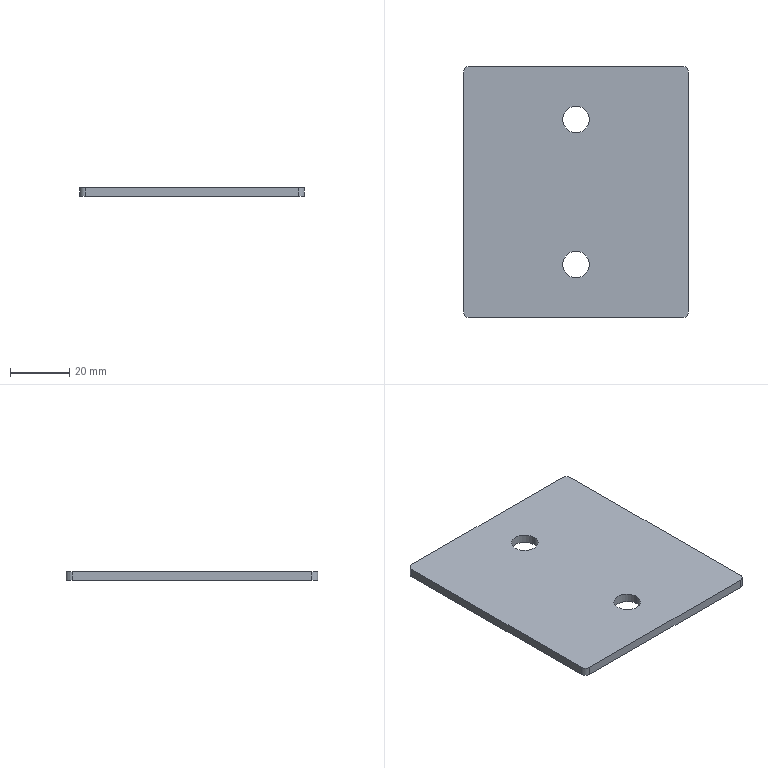Part | SolidWorks | features 3DProfileFeature 1, BreakCorner 1, FlatPattern 1, HoleWzd 1, MirrorPattern 1, SMBaseFlange 1, SheetMetal 1 | 1 solid | 14 faces | box 76 x 85 x 3 mm | volume 18988 mm3 | cylinder 8 | plane 6 | commonest cylinder face diameters 4 x4 9 x4
STEP:
#1=CARTESIAN_POINT('',(4.5,-24.5,-3.));
#2=VERTEX_POINT('',#1);
#3=CARTESIAN_POINT('',(-4.5,-24.5,-3.));
#4=VERTEX_POINT('',#3);
#5=CARTESIAN_POINT('',(0.,-24.5,-3.));
#6=DIRECTION('',(0.,0.,-1.));
#7=DIRECTION('',(-1.,0.,0.));
#8=AXIS2_PLACEMENT_3D('',#5,#6,#7);
#9=CIRCLE('',#8,4.5);
#10=EDGE_CURVE('',#2,#4,#9,.T.);
#11=ORIENTED_EDGE('',*,*,#10,.T.);
#12=CARTESIAN_POINT('',(-4.5,-24.5,0.));
#13=VERTEX_POINT('',#12);
#14=CARTESIAN_POINT('',(-4.5,-24.5,0.));
#15=DIRECTION('',(0.,0.,1.));
#16=VECTOR('',#15,1000.);
#17=LINE('',#14,#16);
#18=EDGE_CURVE('',#4,#13,#17,.T.);
#19=ORIENTED_EDGE('',*,*,#18,.T.);
#20=CARTESIAN_POINT('',(4.5,-24.5,0.));
#21=VERTEX_POINT('',#20);
#22=CARTESIAN_POINT('',(0.,-24.5,0.));
#23=DIRECTION('',(0.,0.,1.));
#24=DIRECTION('',(1.,0.,0.));
#25=AXIS2_PLACEMENT_3D('',#22,#23,#24);
#26=CIRCLE('',#25,4.5);
#27=EDGE_CURVE('',#13,#21,#26,.T.);
#28=ORIENTED_EDGE('',*,*,#27,.T.);
#29=CARTESIAN_POINT('',(4.5,-24.5,0.));
#30=DIRECTION('',(0.,0.,1.));
#31=VECTOR('',#30,1000.);
#32=LINE('',#29,#31);
#33=EDGE_CURVE('',#2,#21,#32,.T.);
#34=ORIENTED_EDGE('',*,*,#33,.F.);
#35=EDGE_LOOP('',(#11,#19,#28,#34));
#36=FACE_OUTER_BOUND('',#35,.T.);
#37=CARTESIAN_POINT('',(0.,-24.5,0.));
#38=DIRECTION('',(0.,0.,1.));
#39=DIRECTION('',(1.,0.,0.));
#40=AXIS2_PLACEMENT_3D('',#37,#38,#39);
#41=CYLINDRICAL_SURFACE('',#40,4.5);
#42=ADVANCED_FACE('',(#36),#41,.F.);
#43=CARTESIAN_POINT('',(4.5,24.5,-3.));
#44=VERTEX_POINT('',#43);
#45=CARTESIAN_POINT('',(-4.5,24.5,-3.));
#46=VERTEX_POINT('',#45);
#47=CARTESIAN_POINT('',(0.,24.5,-3.));
#48=DIRECTION('',(0.,0.,-1.));
#49=DIRECTION('',(-1.,0.,0.));
#50=AXIS2_PLACEMENT_3D('',#47,#48,#49);
#51=CIRCLE('',#50,4.5);
#52=EDGE_CURVE('',#44,#46,#51,.T.);
#53=ORIENTED_EDGE('',*,*,#52,.T.);
#54=CARTESIAN_POINT('',(-4.5,24.5,0.));
#55=VERTEX_POINT('',#54);
#56=CARTESIAN_POINT('',(-4.5,24.5,0.));
#57=DIRECTION('',(0.,0.,1.));
#58=VECTOR('',#57,1000.);
#59=LINE('',#56,#58);
#60=EDGE_CURVE('',#46,#55,#59,.T.);
#61=ORIENTED_EDGE('',*,*,#60,.T.);
#62=CARTESIAN_POINT('',(4.5,24.5,0.));
#63=VERTEX_POINT('',#62);
#64=CARTESIAN_POINT('',(0.,24.5,0.));
#65=DIRECTION('',(0.,0.,1.));
#66=DIRECTION('',(1.,0.,0.));
#67=AXIS2_PLACEMENT_3D('',#64,#65,#66);
#68=CIRCLE('',#67,4.5);
#69=EDGE_CURVE('',#55,#63,#68,.T.);
#70=ORIENTED_EDGE('',*,*,#69,.T.);
#71=CARTESIAN_POINT('',(4.5,24.5,0.));
#72=DIRECTION('',(0.,0.,1.));
#73=VECTOR('',#72,1000.);
#74=LINE('',#71,#73);
#75=EDGE_CURVE('',#44,#63,#74,.T.);
#76=ORIENTED_EDGE('',*,*,#75,.F.);
#77=EDGE_LOOP('',(#53,#61,#70,#76));
#78=FACE_OUTER_BOUND('',#77,.T.);
#79=CARTESIAN_POINT('',(0.,24.5,0.));
#80=DIRECTION('',(0.,0.,1.));
#81=DIRECTION('',(1.,0.,0.));
#82=AXIS2_PLACEMENT_3D('',#79,#80,#81);
#83=CYLINDRICAL_SURFACE('',#82,4.5);
#84=ADVANCED_FACE('',(#78),#83,.F.);
#85=CARTESIAN_POINT('',(0.,-24.5,0.));
#86=DIRECTION('',(0.,0.,1.));
#87=DIRECTION('',(1.,0.,0.));
#88=AXIS2_PLACEMENT_3D('',#85,#86,#87);
#89=CIRCLE('',#88,4.5);
#90=EDGE_CURVE('',#21,#13,#89,.T.);
#91=ORIENTED_EDGE('',*,*,#90,.F.);
#92=ORIENTED_EDGE('',*,*,#27,.F.);
#93=EDGE_LOOP('',(#91,#92));
#94=FACE_BOUND('',#93,.T.);
#95=CARTESIAN_POINT('',(-36.,-42.5,0.));
#96=VERTEX_POINT('',#95);
#97=CARTESIAN_POINT('',(36.,-42.5,0.));
#98=VERTEX_POINT('',#97);
#99=CARTESIAN_POINT('',(-38.,-42.5,0.));
#100=DIRECTION('',(1.,0.,0.));
#101=VECTOR('',#100,1000.);
#102=LINE('',#99,#101);
#103=EDGE_CURVE('',#96,#98,#102,.T.);
#104=ORIENTED_EDGE('',*,*,#103,.T.);
#105=CARTESIAN_POINT('',(38.,-40.5,0.));
#106=VERTEX_POINT('',#105);
#107=CARTESIAN_POINT('',(36.,-40.5,0.));
#108=DIRECTION('',(0.,0.,1.));
#109=DIRECTION('',(-1.,0.,0.));
#110=AXIS2_PLACEMENT_3D('',#107,#108,#109);
#111=CIRCLE('',#110,2.);
#112=EDGE_CURVE('',#98,#106,#111,.T.);
#113=ORIENTED_EDGE('',*,*,#112,.T.);
#114=CARTESIAN_POINT('',(38.,40.5,0.));
#115=VERTEX_POINT('',#114);
#116=CARTESIAN_POINT('',(38.,-42.5,0.));
#117=DIRECTION('',(0.,1.,0.));
#118=VECTOR('',#117,1000.);
#119=LINE('',#116,#118);
#120=EDGE_CURVE('',#106,#115,#119,.T.);
#121=ORIENTED_EDGE('',*,*,#120,.T.);
#122=CARTESIAN_POINT('',(36.,42.5,0.));
#123=VERTEX_POINT('',#122);
#124=CARTESIAN_POINT('',(36.,40.5,0.));
#125=DIRECTION('',(0.,0.,1.));
#126=DIRECTION('',(-1.,0.,0.));
#127=AXIS2_PLACEMENT_3D('',#124,#125,#126);
#128=CIRCLE('',#127,2.);
#129=EDGE_CURVE('',#115,#123,#128,.T.);
#130=ORIENTED_EDGE('',*,*,#129,.T.);
#131=CARTESIAN_POINT('',(-36.,42.5,0.));
#132=VERTEX_POINT('',#131);
#133=CARTESIAN_POINT('',(-38.,42.5,0.));
#134=DIRECTION('',(-1.,0.,0.));
#135=VECTOR('',#134,1000.);
#136=LINE('',#133,#135);
#137=EDGE_CURVE('',#123,#132,#136,.T.);
#138=ORIENTED_EDGE('',*,*,#137,.T.);
#139=CARTESIAN_POINT('',(-38.,40.5,0.));
#140=VERTEX_POINT('',#139);
#141=CARTESIAN_POINT('',(-36.,40.5,0.));
#142=DIRECTION('',(0.,0.,1.));
#143=DIRECTION('',(-1.,0.,0.));
#144=AXIS2_PLACEMENT_3D('',#141,#142,#143);
#145=CIRCLE('',#144,2.);
#146=EDGE_CURVE('',#132,#140,#145,.T.);
#147=ORIENTED_EDGE('',*,*,#146,.T.);
#148=CARTESIAN_POINT('',(-38.,-40.5,0.));
#149=VERTEX_POINT('',#148);
#150=CARTESIAN_POINT('',(-38.,-42.5,0.));
#151=DIRECTION('',(0.,-1.,0.));
#152=VECTOR('',#151,1000.);
#153=LINE('',#150,#152);
#154=EDGE_CURVE('',#140,#149,#153,.T.);
#155=ORIENTED_EDGE('',*,*,#154,.T.);
#156=CARTESIAN_POINT('',(-36.,-40.5,0.));
#157=DIRECTION('',(0.,0.,1.));
#158=DIRECTION('',(-1.,0.,0.));
#159=AXIS2_PLACEMENT_3D('',#156,#157,#158);
#160=CIRCLE('',#159,2.);
#161=EDGE_CURVE('',#149,#96,#160,.T.);
#162=ORIENTED_EDGE('',*,*,#161,.T.);
#163=EDGE_LOOP('',(#104,#113,#121,#130,#138,#147,#155,#162));
#164=FACE_OUTER_BOUND('',#163,.T.);
#165=CARTESIAN_POINT('',(0.,24.5,0.));
#166=DIRECTION('',(0.,0.,1.));
#167=DIRECTION('',(1.,0.,0.));
#168=AXIS2_PLACEMENT_3D('',#165,#166,#167);
#169=CIRCLE('',#168,4.5);
#170=EDGE_CURVE('',#63,#55,#169,.T.);
#171=ORIENTED_EDGE('',*,*,#170,.F.);
#172=ORIENTED_EDGE('',*,*,#69,.F.);
#173=EDGE_LOOP('',(#171,#172));
#174=FACE_BOUND('',#173,.T.);
#175=CARTESIAN_POINT('',(0.,0.,0.));
#176=DIRECTION('',(0.,0.,-1.));
#177=DIRECTION('',(-1.,0.,0.));
#178=AXIS2_PLACEMENT_3D('',#175,#176,#177);
#179=PLANE('',#178);
#180=ADVANCED_FACE('',(#94,#164,#174),#179,.F.);
#181=ORIENTED_EDGE('',*,*,#120,.F.);
#182=CARTESIAN_POINT('',(38.,-40.5,-3.));
#183=VERTEX_POINT('',#182);
#184=CARTESIAN_POINT('',(38.,-40.5,-3.));
#185=DIRECTION('',(0.,0.,-1.));
#186=VECTOR('',#185,1000.);
#187=LINE('',#184,#186);
#188=EDGE_CURVE('',#106,#183,#187,.T.);
#189=ORIENTED_EDGE('',*,*,#188,.T.);
#190=CARTESIAN_POINT('',(38.,40.5,-3.));
#191=VERTEX_POINT('',#190);
#192=CARTESIAN_POINT('',(38.,-42.5,-3.));
#193=DIRECTION('',(0.,1.,0.));
#194=VECTOR('',#193,1000.);
#195=LINE('',#192,#194);
#196=EDGE_CURVE('',#183,#191,#195,.T.);
#197=ORIENTED_EDGE('',*,*,#196,.T.);
#198=CARTESIAN_POINT('',(38.,40.5,-3.));
#199=DIRECTION('',(0.,0.,1.));
#200=VECTOR('',#199,1000.);
#201=LINE('',#198,#200);
#202=EDGE_CURVE('',#191,#115,#201,.T.);
#203=ORIENTED_EDGE('',*,*,#202,.T.);
#204=EDGE_LOOP('',(#181,#189,#197,#203));
#205=FACE_OUTER_BOUND('',#204,.T.);
#206=CARTESIAN_POINT('',(38.,-42.5,-3.));
#207=DIRECTION('',(1.,0.,0.));
#208=DIRECTION('',(0.,0.,-1.));
#209=AXIS2_PLACEMENT_3D('',#206,#207,#208);
#210=PLANE('',#209);
#211=ADVANCED_FACE('',(#205),#210,.T.);
#212=CARTESIAN_POINT('',(-36.,-42.5,-3.));
#213=VERTEX_POINT('',#212);
#214=CARTESIAN_POINT('',(36.,-42.5,-3.));
#215=VERTEX_POINT('',#214);
#216=CARTESIAN_POINT('',(-38.,-42.5,-3.));
#217=DIRECTION('',(1.,0.,0.));
#218=VECTOR('',#217,1000.);
#219=LINE('',#216,#218);
#220=EDGE_CURVE('',#213,#215,#219,.T.);
#221=ORIENTED_EDGE('',*,*,#220,.T.);
#222=CARTESIAN_POINT('',(36.,-42.5,-3.));
#223=DIRECTION('',(0.,0.,1.));
#224=VECTOR('',#223,1000.);
#225=LINE('',#222,#224);
#226=EDGE_CURVE('',#215,#98,#225,.T.);
#227=ORIENTED_EDGE('',*,*,#226,.T.);
#228=ORIENTED_EDGE('',*,*,#103,.F.);
#229=CARTESIAN_POINT('',(-36.,-42.5,-3.));
#230=DIRECTION('',(0.,0.,-1.));
#231=VECTOR('',#230,1000.);
#232=LINE('',#229,#231);
#233=EDGE_CURVE('',#96,#213,#232,.T.);
#234=ORIENTED_EDGE('',*,*,#233,.T.);
#235=EDGE_LOOP('',(#221,#227,#228,#234));
#236=FACE_OUTER_BOUND('',#235,.T.);
#237=CARTESIAN_POINT('',(-38.,-42.5,-3.));
#238=DIRECTION('',(0.,-1.,0.));
#239=DIRECTION('',(0.,0.,-1.));
#240=AXIS2_PLACEMENT_3D('',#237,#238,#239);
#241=PLANE('',#240);
#242=ADVANCED_FACE('',(#236),#241,.T.);
#243=CARTESIAN_POINT('',(-38.,40.5,-3.));
#244=VERTEX_POINT('',#243);
#245=CARTESIAN_POINT('',(-38.,-40.5,-3.));
#246=VERTEX_POINT('',#245);
#247=CARTESIAN_POINT('',(-38.,-42.5,-3.));
#248=DIRECTION('',(0.,-1.,0.));
#249=VECTOR('',#248,1000.);
#250=LINE('',#247,#249);
#251=EDGE_CURVE('',#244,#246,#250,.T.);
#252=ORIENTED_EDGE('',*,*,#251,.T.);
#253=CARTESIAN_POINT('',(-38.,-40.5,-3.));
#254=DIRECTION('',(0.,0.,1.));
#255=VECTOR('',#254,1000.);
#256=LINE('',#253,#255);
#257=EDGE_CURVE('',#246,#149,#256,.T.);
#258=ORIENTED_EDGE('',*,*,#257,.T.);
#259=ORIENTED_EDGE('',*,*,#154,.F.);
#260=CARTESIAN_POINT('',(-38.,40.5,-3.));
#261=DIRECTION('',(0.,0.,-1.));
#262=VECTOR('',#261,1000.);
#263=LINE('',#260,#262);
#264=EDGE_CURVE('',#140,#244,#263,.T.);
#265=ORIENTED_EDGE('',*,*,#264,.T.);
#266=EDGE_LOOP('',(#252,#258,#259,#265));
#267=FACE_OUTER_BOUND('',#266,.T.);
#268=CARTESIAN_POINT('',(-38.,-42.5,-3.));
#269=DIRECTION('',(-1.,0.,0.));
#270=DIRECTION('',(0.,0.,1.));
#271=AXIS2_PLACEMENT_3D('',#268,#269,#270);
#272=PLANE('',#271);
#273=ADVANCED_FACE('',(#267),#272,.T.);
#274=CARTESIAN_POINT('',(36.,42.5,-3.));
#275=VERTEX_POINT('',#274);
#276=CARTESIAN_POINT('',(-36.,42.5,-3.));
#277=VERTEX_POINT('',#276);
#278=CARTESIAN_POINT('',(-38.,42.5,-3.));
#279=DIRECTION('',(-1.,0.,0.));
#280=VECTOR('',#279,1000.);
#281=LINE('',#278,#280);
#282=EDGE_CURVE('',#275,#277,#281,.T.);
#283=ORIENTED_EDGE('',*,*,#282,.T.);
#284=CARTESIAN_POINT('',(-36.,42.5,-3.));
#285=DIRECTION('',(0.,0.,1.));
#286=VECTOR('',#285,1000.);
#287=LINE('',#284,#286);
#288=EDGE_CURVE('',#277,#132,#287,.T.);
#289=ORIENTED_EDGE('',*,*,#288,.T.);
#290=ORIENTED_EDGE('',*,*,#137,.F.);
#291=CARTESIAN_POINT('',(36.,42.5,-3.));
#292=DIRECTION('',(0.,0.,-1.));
#293=VECTOR('',#292,1000.);
#294=LINE('',#291,#293);
#295=EDGE_CURVE('',#123,#275,#294,.T.);
#296=ORIENTED_EDGE('',*,*,#295,.T.);
#297=EDGE_LOOP('',(#283,#289,#290,#296));
#298=FACE_OUTER_BOUND('',#297,.T.);
#299=CARTESIAN_POINT('',(-38.,42.5,-3.));
#300=DIRECTION('',(0.,1.,0.));
#301=DIRECTION('',(0.,0.,1.));
#302=AXIS2_PLACEMENT_3D('',#299,#300,#301);
#303=PLANE('',#302);
#304=ADVANCED_FACE('',(#298),#303,.T.);
#305=ORIENTED_EDGE('',*,*,#10,.F.);
#306=CARTESIAN_POINT('',(0.,-24.5,-3.));
#307=DIRECTION('',(0.,0.,-1.));
#308=DIRECTION('',(-1.,0.,0.));
#309=AXIS2_PLACEMENT_3D('',#306,#307,#308);
#310=CIRCLE('',#309,4.5);
#311=EDGE_CURVE('',#4,#2,#310,.T.);
#312=ORIENTED_EDGE('',*,*,#311,.F.);
#313=EDGE_LOOP('',(#305,#312));
#314=FACE_BOUND('',#313,.T.);
#315=ORIENTED_EDGE('',*,*,#52,.F.);
#316=CARTESIAN_POINT('',(0.,24.5,-3.));
#317=DIRECTION('',(0.,0.,-1.));
#318=DIRECTION('',(-1.,0.,0.));
#319=AXIS2_PLACEMENT_3D('',#316,#317,#318);
#320=CIRCLE('',#319,4.5);
#321=EDGE_CURVE('',#46,#44,#320,.T.);
#322=ORIENTED_EDGE('',*,*,#321,.F.);
#323=EDGE_LOOP('',(#315,#322));
#324=FACE_BOUND('',#323,.T.);
#325=ORIENTED_EDGE('',*,*,#196,.F.);
#326=CARTESIAN_POINT('',(36.,-40.5,-3.));
#327=DIRECTION('',(0.,0.,-1.));
#328=DIRECTION('',(-1.,0.,0.));
#329=AXIS2_PLACEMENT_3D('',#326,#327,#328);
#330=CIRCLE('',#329,2.);
#331=EDGE_CURVE('',#183,#215,#330,.T.);
#332=ORIENTED_EDGE('',*,*,#331,.T.);
#333=ORIENTED_EDGE('',*,*,#220,.F.);
#334=CARTESIAN_POINT('',(-36.,-40.5,-3.));
#335=DIRECTION('',(0.,0.,-1.));
#336=DIRECTION('',(-1.,0.,0.));
#337=AXIS2_PLACEMENT_3D('',#334,#335,#336);
#338=CIRCLE('',#337,2.);
#339=EDGE_CURVE('',#213,#246,#338,.T.);
#340=ORIENTED_EDGE('',*,*,#339,.T.);
#341=ORIENTED_EDGE('',*,*,#251,.F.);
#342=CARTESIAN_POINT('',(-36.,40.5,-3.));
#343=DIRECTION('',(0.,0.,-1.));
#344=DIRECTION('',(-1.,0.,0.));
#345=AXIS2_PLACEMENT_3D('',#342,#343,#344);
#346=CIRCLE('',#345,2.);
#347=EDGE_CURVE('',#244,#277,#346,.T.);
#348=ORIENTED_EDGE('',*,*,#347,.T.);
#349=ORIENTED_EDGE('',*,*,#282,.F.);
#350=CARTESIAN_POINT('',(36.,40.5,-3.));
#351=DIRECTION('',(0.,0.,-1.));
#352=DIRECTION('',(-1.,0.,0.));
#353=AXIS2_PLACEMENT_3D('',#350,#351,#352);
#354=CIRCLE('',#353,2.);
#355=EDGE_CURVE('',#275,#191,#354,.T.);
#356=ORIENTED_EDGE('',*,*,#355,.T.);
#357=EDGE_LOOP('',(#325,#332,#333,#340,#341,#348,#349,#356));
#358=FACE_OUTER_BOUND('',#357,.T.);
#359=CARTESIAN_POINT('',(0.,0.,-3.));
#360=DIRECTION('',(0.,0.,-1.));
#361=DIRECTION('',(-1.,0.,0.));
#362=AXIS2_PLACEMENT_3D('',#359,#360,#361);
#363=PLANE('',#362);
#364=ADVANCED_FACE('',(#314,#324,#358),#363,.T.);
#365=ORIENTED_EDGE('',*,*,#331,.F.);
#366=ORIENTED_EDGE('',*,*,#188,.F.);
#367=ORIENTED_EDGE('',*,*,#112,.F.);
#368=ORIENTED_EDGE('',*,*,#226,.F.);
#369=EDGE_LOOP('',(#365,#366,#367,#368));
#370=FACE_OUTER_BOUND('',#369,.T.);
#371=CARTESIAN_POINT('',(36.,-40.5,-3.));
#372=DIRECTION('',(0.,0.,1.));
#373=DIRECTION('',(1.,0.,0.));
#374=AXIS2_PLACEMENT_3D('',#371,#372,#373);
#375=CYLINDRICAL_SURFACE('',#374,2.);
#376=ADVANCED_FACE('',(#370),#375,.T.);
#377=ORIENTED_EDGE('',*,*,#339,.F.);
#378=ORIENTED_EDGE('',*,*,#233,.F.);
#379=ORIENTED_EDGE('',*,*,#161,.F.);
#380=ORIENTED_EDGE('',*,*,#257,.F.);
#381=EDGE_LOOP('',(#377,#378,#379,#380));
#382=FACE_OUTER_BOUND('',#381,.T.);
#383=CARTESIAN_POINT('',(-36.,-40.5,-3.));
#384=DIRECTION('',(0.,0.,1.));
#385=DIRECTION('',(1.,0.,0.));
#386=AXIS2_PLACEMENT_3D('',#383,#384,#385);
#387=CYLINDRICAL_SURFACE('',#386,2.);
#388=ADVANCED_FACE('',(#382),#387,.T.);
#389=ORIENTED_EDGE('',*,*,#347,.F.);
#390=ORIENTED_EDGE('',*,*,#264,.F.);
#391=ORIENTED_EDGE('',*,*,#146,.F.);
#392=ORIENTED_EDGE('',*,*,#288,.F.);
#393=EDGE_LOOP('',(#389,#390,#391,#392));
#394=FACE_OUTER_BOUND('',#393,.T.);
#395=CARTESIAN_POINT('',(-36.,40.5,-3.));
#396=DIRECTION('',(0.,0.,1.));
#397=DIRECTION('',(1.,0.,0.));
#398=AXIS2_PLACEMENT_3D('',#395,#396,#397);
#399=CYLINDRICAL_SURFACE('',#398,2.);
#400=ADVANCED_FACE('',(#394),#399,.T.);
#401=ORIENTED_EDGE('',*,*,#355,.F.);
#402=ORIENTED_EDGE('',*,*,#295,.F.);
#403=ORIENTED_EDGE('',*,*,#129,.F.);
#404=ORIENTED_EDGE('',*,*,#202,.F.);
#405=EDGE_LOOP('',(#401,#402,#403,#404));
#406=FACE_OUTER_BOUND('',#405,.T.);
#407=CARTESIAN_POINT('',(36.,40.5,-3.));
#408=DIRECTION('',(0.,0.,1.));
#409=DIRECTION('',(1.,0.,0.));
#410=AXIS2_PLACEMENT_3D('',#407,#408,#409);
#411=CYLINDRICAL_SURFACE('',#410,2.);
#412=ADVANCED_FACE('',(#406),#411,.T.);
#413=ORIENTED_EDGE('',*,*,#60,.F.);
#414=ORIENTED_EDGE('',*,*,#321,.T.);
#415=ORIENTED_EDGE('',*,*,#75,.T.);
#416=ORIENTED_EDGE('',*,*,#170,.T.);
#417=EDGE_LOOP('',(#413,#414,#415,#416));
#418=FACE_OUTER_BOUND('',#417,.T.);
#419=CARTESIAN_POINT('',(0.,24.5,0.));
#420=DIRECTION('',(0.,0.,1.));
#421=DIRECTION('',(1.,0.,0.));
#422=AXIS2_PLACEMENT_3D('',#419,#420,#421);
#423=CYLINDRICAL_SURFACE('',#422,4.5);
#424=ADVANCED_FACE('',(#418),#423,.F.);
#425=ORIENTED_EDGE('',*,*,#18,.F.);
#426=ORIENTED_EDGE('',*,*,#311,.T.);
#427=ORIENTED_EDGE('',*,*,#33,.T.);
#428=ORIENTED_EDGE('',*,*,#90,.T.);
#429=EDGE_LOOP('',(#425,#426,#427,#428));
#430=FACE_OUTER_BOUND('',#429,.T.);
#431=CARTESIAN_POINT('',(0.,-24.5,0.));
#432=DIRECTION('',(0.,0.,1.));
#433=DIRECTION('',(1.,0.,0.));
#434=AXIS2_PLACEMENT_3D('',#431,#432,#433);
#435=CYLINDRICAL_SURFACE('',#434,4.5);
#436=ADVANCED_FACE('',(#430),#435,.F.);
#437=CLOSED_SHELL('',(#42,#84,#180,#211,#242,#273,#304,#364,#376,#388,#400,#412,#424,#436));
#438=MANIFOLD_SOLID_BREP('',#437);
#439=CARTESIAN_POINT('',(0.,0.,0.));
#440=DIRECTION('',(0.,0.,1.));
#441=DIRECTION('',(1.,0.,0.));
#442=AXIS2_PLACEMENT_3D('',#439,#440,#441);
#443=(LENGTH_UNIT()NAMED_UNIT(*)SI_UNIT(.MILLI.,.METRE.));
#444=UNCERTAINTY_MEASURE_WITH_UNIT(LENGTH_MEASURE(0.00001),#443,'','');
#445=(NAMED_UNIT(*)PLANE_ANGLE_UNIT()SI_UNIT($,.RADIAN.));
#446=(NAMED_UNIT(*)SI_UNIT($,.STERADIAN.)SOLID_ANGLE_UNIT());
#447=(GEOMETRIC_REPRESENTATION_CONTEXT(3)GLOBAL_UNCERTAINTY_ASSIGNED_CONTEXT((#444))GLOBAL_UNIT_ASSIGNED_CONTEXT((#443,#445,#446))REPRESENTATION_CONTEXT('',''));
#448=ADVANCED_BREP_SHAPE_REPRESENTATION('',(#438,#442),#447);